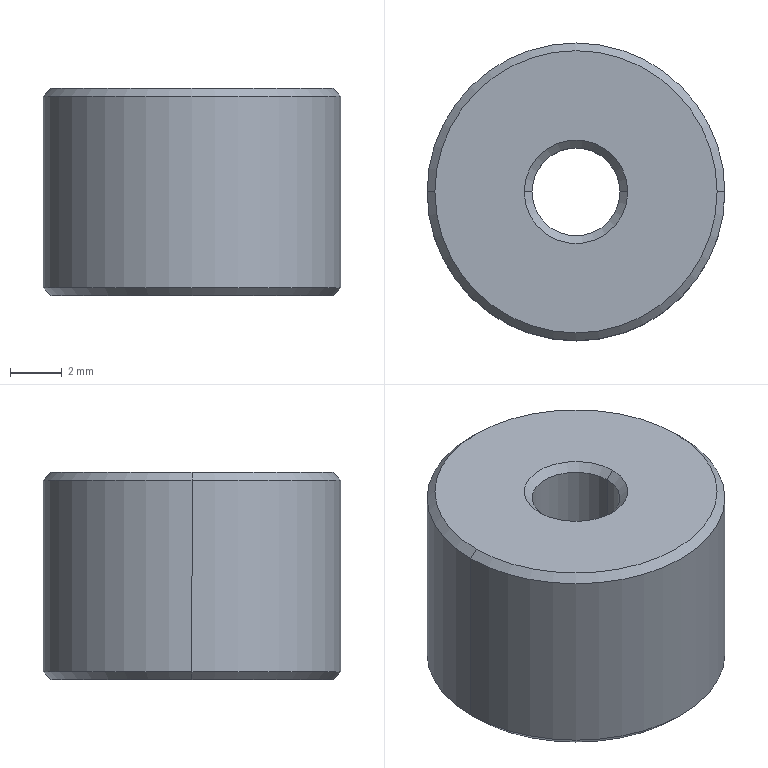Part | STEP file | Guide post cap | 1 solid | 17 faces | box 11.5 x 11.5 x 8 mm | volume 657.251 mm3 | cone 8 | cylinder 6 | plane 3 | commonest cylinder face diameters 3.4 x2 6.5 x2 11.5 x2
STEP:
#1=CARTESIAN_POINT('',(0.,0.,0.));
#2=DIRECTION('',(0.,0.,1.));
#3=DIRECTION('',(1.,0.,0.));
#4=AXIS2_PLACEMENT_3D('',#1,#2,#3);
#5=CARTESIAN_POINT('',(-5.75,0.,7.7));
#6=VERTEX_POINT('',#5);
#7=CARTESIAN_POINT('',(5.75,0.,7.7));
#8=VERTEX_POINT('',#7);
#9=CARTESIAN_POINT('',(0.,0.,7.7));
#10=DIRECTION('',(0.,0.,-1.));
#11=DIRECTION('',(-1.,0.,0.));
#12=AXIS2_PLACEMENT_3D('',#9,#10,#11);
#13=CIRCLE('',#12,5.75);
#14=CARTESIAN_POINT('',(0.,0.,8.));
#15=DIRECTION('',(0.,0.,-1.));
#16=DIRECTION('',(-1.,0.,0.));
#17=AXIS2_PLACEMENT_3D('',#14,#15,#16);
#18=CYLINDRICAL_SURFACE('',#17,5.75);
#19=CARTESIAN_POINT('',(0.,0.3));
#20=DIRECTION('',(1.,0.));
#21=VECTOR('',#20,1.);
#22=LINE('',#19,#21);
#23=(GEOMETRIC_REPRESENTATION_CONTEXT(2)PARAMETRIC_REPRESENTATION_CONTEXT()REPRESENTATION_CONTEXT('',''));
#24=DEFINITIONAL_REPRESENTATION('',(#22),#23);
#25=PCURVE('',#18,#24);
#26=CARTESIAN_POINT('',(0.,0.,7.7));
#27=DIRECTION('',(0.,0.,-1.));
#28=DIRECTION('',(-1.,0.,0.));
#29=AXIS2_PLACEMENT_3D('',#26,#27,#28);
#30=CONICAL_SURFACE('',#29,5.75,0.7854);
#31=CARTESIAN_POINT('',(0.,0.));
#32=DIRECTION('',(1.,0.));
#33=VECTOR('',#32,1.);
#34=LINE('',#31,#33);
#35=(GEOMETRIC_REPRESENTATION_CONTEXT(2)PARAMETRIC_REPRESENTATION_CONTEXT()REPRESENTATION_CONTEXT('',''));
#36=DEFINITIONAL_REPRESENTATION('',(#34),#35);
#37=PCURVE('',#30,#36);
#38=SURFACE_CURVE('',#13,(#25,#37),.PCURVE_S1.);
#39=EDGE_CURVE('',#6,#8,#38,.T.);
#40=ORIENTED_EDGE('',*,*,#39,.T.);
#41=CARTESIAN_POINT('',(5.75,0.,0.3));
#42=VERTEX_POINT('',#41);
#43=CARTESIAN_POINT('',(5.75,0.,8.));
#44=DIRECTION('',(0.,0.,-1.));
#45=VECTOR('',#44,1.);
#46=LINE('',#43,#45);
#47=CARTESIAN_POINT('',(3.142,0.));
#48=DIRECTION('',(0.,1.));
#49=VECTOR('',#48,1.);
#50=LINE('',#47,#49);
#51=(GEOMETRIC_REPRESENTATION_CONTEXT(2)PARAMETRIC_REPRESENTATION_CONTEXT()REPRESENTATION_CONTEXT('',''));
#52=DEFINITIONAL_REPRESENTATION('',(#50),#51);
#53=PCURVE('',#18,#52);
#54=CARTESIAN_POINT('',(0.,0.,8.));
#55=DIRECTION('',(0.,0.,-1.));
#56=DIRECTION('',(-1.,0.,0.));
#57=AXIS2_PLACEMENT_3D('',#54,#55,#56);
#58=CYLINDRICAL_SURFACE('',#57,5.75);
#59=CARTESIAN_POINT('',(3.142,0.));
#60=DIRECTION('',(0.,1.));
#61=VECTOR('',#60,1.);
#62=LINE('',#59,#61);
#63=(GEOMETRIC_REPRESENTATION_CONTEXT(2)PARAMETRIC_REPRESENTATION_CONTEXT()REPRESENTATION_CONTEXT('',''));
#64=DEFINITIONAL_REPRESENTATION('',(#62),#63);
#65=PCURVE('',#58,#64);
#66=SURFACE_CURVE('',#46,(#53,#65),.PCURVE_S1.);
#67=EDGE_CURVE('',#8,#42,#66,.T.);
#68=ORIENTED_EDGE('',*,*,#67,.T.);
#69=CARTESIAN_POINT('',(-5.75,0.,0.3));
#70=VERTEX_POINT('',#69);
#71=CARTESIAN_POINT('',(0.,0.,0.3));
#72=DIRECTION('',(0.,0.,1.));
#73=DIRECTION('',(-1.,0.,0.));
#74=AXIS2_PLACEMENT_3D('',#71,#72,#73);
#75=CIRCLE('',#74,5.75);
#76=CARTESIAN_POINT('',(6.283,7.7));
#77=DIRECTION('',(-1.,0.));
#78=VECTOR('',#77,1.);
#79=LINE('',#76,#78);
#80=(GEOMETRIC_REPRESENTATION_CONTEXT(2)PARAMETRIC_REPRESENTATION_CONTEXT()REPRESENTATION_CONTEXT('',''));
#81=DEFINITIONAL_REPRESENTATION('',(#79),#80);
#82=PCURVE('',#18,#81);
#83=CARTESIAN_POINT('',(0.,0.,0.3));
#84=DIRECTION('',(0.,0.,1.));
#85=DIRECTION('',(1.,0.,0.));
#86=AXIS2_PLACEMENT_3D('',#83,#84,#85);
#87=CONICAL_SURFACE('',#86,5.75,0.7854);
#88=CARTESIAN_POINT('',(-3.142,0.));
#89=DIRECTION('',(1.,0.));
#90=VECTOR('',#89,1.);
#91=LINE('',#88,#90);
#92=(GEOMETRIC_REPRESENTATION_CONTEXT(2)PARAMETRIC_REPRESENTATION_CONTEXT()REPRESENTATION_CONTEXT('',''));
#93=DEFINITIONAL_REPRESENTATION('',(#91),#92);
#94=PCURVE('',#87,#93);
#95=SURFACE_CURVE('',#75,(#82,#94),.PCURVE_S1.);
#96=EDGE_CURVE('',#42,#70,#95,.T.);
#97=ORIENTED_EDGE('',*,*,#96,.T.);
#98=CARTESIAN_POINT('',(-5.75,0.,8.));
#99=DIRECTION('',(0.,0.,-1.));
#100=VECTOR('',#99,1.);
#101=LINE('',#98,#100);
#102=CARTESIAN_POINT('',(0.,0.));
#103=DIRECTION('',(0.,1.));
#104=VECTOR('',#103,1.);
#105=LINE('',#102,#104);
#106=(GEOMETRIC_REPRESENTATION_CONTEXT(2)PARAMETRIC_REPRESENTATION_CONTEXT()REPRESENTATION_CONTEXT('',''));
#107=DEFINITIONAL_REPRESENTATION('',(#105),#106);
#108=PCURVE('',#18,#107);
#109=CARTESIAN_POINT('',(6.283,0.));
#110=DIRECTION('',(0.,1.));
#111=VECTOR('',#110,1.);
#112=LINE('',#109,#111);
#113=(GEOMETRIC_REPRESENTATION_CONTEXT(2)PARAMETRIC_REPRESENTATION_CONTEXT()REPRESENTATION_CONTEXT('',''));
#114=DEFINITIONAL_REPRESENTATION('',(#112),#113);
#115=PCURVE('',#58,#114);
#116=SURFACE_CURVE('',#101,(#108,#115),.PCURVE_S1.);
#117=EDGE_CURVE('',#6,#70,#116,.T.);
#118=ORIENTED_EDGE('',*,*,#117,.F.);
#119=EDGE_LOOP('',(#40,#68,#97,#118));
#120=FACE_BOUND('',#119,.T.);
#121=ADVANCED_FACE('',(#120),#18,.T.);
#122=CARTESIAN_POINT('',(5.45,0.,0.));
#123=VERTEX_POINT('',#122);
#124=CARTESIAN_POINT('',(-5.45,0.,0.));
#125=VERTEX_POINT('',#124);
#126=CARTESIAN_POINT('',(0.,0.,0.));
#127=DIRECTION('',(0.,0.,1.));
#128=DIRECTION('',(1.,0.,0.));
#129=AXIS2_PLACEMENT_3D('',#126,#127,#128);
#130=CIRCLE('',#129,5.45);
#131=CARTESIAN_POINT('',(0.,-0.3));
#132=DIRECTION('',(1.,0.));
#133=VECTOR('',#132,1.);
#134=LINE('',#131,#133);
#135=(GEOMETRIC_REPRESENTATION_CONTEXT(2)PARAMETRIC_REPRESENTATION_CONTEXT()REPRESENTATION_CONTEXT('',''));
#136=DEFINITIONAL_REPRESENTATION('',(#134),#135);
#137=PCURVE('',#87,#136);
#138=CARTESIAN_POINT('',(0.,0.,0.));
#139=DIRECTION('',(0.,0.,1.));
#140=DIRECTION('',(1.,0.,0.));
#141=AXIS2_PLACEMENT_3D('',#138,#139,#140);
#142=PLANE('',#141);
#143=CARTESIAN_POINT('',(0.,0.));
#144=DIRECTION('',(1.,0.));
#145=AXIS2_PLACEMENT_2D('',#143,#144);
#146=CIRCLE('',#145,5.45);
#147=(GEOMETRIC_REPRESENTATION_CONTEXT(2)PARAMETRIC_REPRESENTATION_CONTEXT()REPRESENTATION_CONTEXT('',''));
#148=DEFINITIONAL_REPRESENTATION('',(#146),#147);
#149=PCURVE('',#142,#148);
#150=SURFACE_CURVE('',#130,(#137,#149),.PCURVE_S1.);
#151=EDGE_CURVE('',#123,#125,#150,.T.);
#152=ORIENTED_EDGE('',*,*,#151,.T.);
#153=CARTESIAN_POINT('',(-5.75,0.,0.3));
#154=DIRECTION('',(-0.7071,0.,0.7071));
#155=VECTOR('',#154,1.);
#156=LINE('',#153,#155);
#157=CARTESIAN_POINT('',(3.142,0.));
#158=DIRECTION('',(0.,1.));
#159=VECTOR('',#158,1.);
#160=LINE('',#157,#159);
#161=(GEOMETRIC_REPRESENTATION_CONTEXT(2)PARAMETRIC_REPRESENTATION_CONTEXT()REPRESENTATION_CONTEXT('',''));
#162=DEFINITIONAL_REPRESENTATION('',(#160),#161);
#163=PCURVE('',#87,#162);
#164=CARTESIAN_POINT('',(0.,0.,0.3));
#165=DIRECTION('',(0.,0.,1.));
#166=DIRECTION('',(1.,0.,0.));
#167=AXIS2_PLACEMENT_3D('',#164,#165,#166);
#168=CONICAL_SURFACE('',#167,5.75,0.7854);
#169=CARTESIAN_POINT('',(3.142,0.));
#170=DIRECTION('',(0.,1.));
#171=VECTOR('',#170,1.);
#172=LINE('',#169,#171);
#173=(GEOMETRIC_REPRESENTATION_CONTEXT(2)PARAMETRIC_REPRESENTATION_CONTEXT()REPRESENTATION_CONTEXT('',''));
#174=DEFINITIONAL_REPRESENTATION('',(#172),#173);
#175=PCURVE('',#168,#174);
#176=SURFACE_CURVE('',#156,(#163,#175),.PCURVE_S1.);
#177=EDGE_CURVE('',#125,#70,#176,.T.);
#178=ORIENTED_EDGE('',*,*,#177,.T.);
#179=ORIENTED_EDGE('',*,*,#96,.F.);
#180=CARTESIAN_POINT('',(5.75,0.,0.3));
#181=DIRECTION('',(0.7071,0.,0.7071));
#182=VECTOR('',#181,1.);
#183=LINE('',#180,#182);
#184=CARTESIAN_POINT('',(0.,0.));
#185=DIRECTION('',(0.,1.));
#186=VECTOR('',#185,1.);
#187=LINE('',#184,#186);
#188=(GEOMETRIC_REPRESENTATION_CONTEXT(2)PARAMETRIC_REPRESENTATION_CONTEXT()REPRESENTATION_CONTEXT('',''));
#189=DEFINITIONAL_REPRESENTATION('',(#187),#188);
#190=PCURVE('',#87,#189);
#191=CARTESIAN_POINT('',(6.283,0.));
#192=DIRECTION('',(0.,1.));
#193=VECTOR('',#192,1.);
#194=LINE('',#191,#193);
#195=(GEOMETRIC_REPRESENTATION_CONTEXT(2)PARAMETRIC_REPRESENTATION_CONTEXT()REPRESENTATION_CONTEXT('',''));
#196=DEFINITIONAL_REPRESENTATION('',(#194),#195);
#197=PCURVE('',#168,#196);
#198=SURFACE_CURVE('',#183,(#190,#197),.PCURVE_S1.);
#199=EDGE_CURVE('',#123,#42,#198,.T.);
#200=ORIENTED_EDGE('',*,*,#199,.F.);
#201=EDGE_LOOP('',(#152,#178,#179,#200));
#202=FACE_BOUND('',#201,.T.);
#203=ADVANCED_FACE('',(#202),#87,.T.);
#204=CARTESIAN_POINT('',(-5.45,0.,8.));
#205=VERTEX_POINT('',#204);
#206=CARTESIAN_POINT('',(5.45,0.,8.));
#207=VERTEX_POINT('',#206);
#208=CARTESIAN_POINT('',(0.,0.,8.));
#209=DIRECTION('',(0.,0.,-1.));
#210=DIRECTION('',(-1.,0.,0.));
#211=AXIS2_PLACEMENT_3D('',#208,#209,#210);
#212=CIRCLE('',#211,5.45);
#213=CARTESIAN_POINT('',(0.,-0.3));
#214=DIRECTION('',(1.,0.));
#215=VECTOR('',#214,1.);
#216=LINE('',#213,#215);
#217=(GEOMETRIC_REPRESENTATION_CONTEXT(2)PARAMETRIC_REPRESENTATION_CONTEXT()REPRESENTATION_CONTEXT('',''));
#218=DEFINITIONAL_REPRESENTATION('',(#216),#217);
#219=PCURVE('',#30,#218);
#220=CARTESIAN_POINT('',(0.,0.,8.));
#221=DIRECTION('',(0.,0.,1.));
#222=DIRECTION('',(1.,0.,0.));
#223=AXIS2_PLACEMENT_3D('',#220,#221,#222);
#224=PLANE('',#223);
#225=CARTESIAN_POINT('',(-5.45,0.));
#226=CARTESIAN_POINT('',(-5.45,9.44));
#227=CARTESIAN_POINT('',(2.725,4.72));
#228=CARTESIAN_POINT('',(10.9,0.));
#229=CARTESIAN_POINT('',(2.725,-4.72));
#230=CARTESIAN_POINT('',(-5.45,-9.44));
#231=CARTESIAN_POINT('',(-5.45,0.));
#232=(BOUNDED_CURVE()B_SPLINE_CURVE(2,(#225,#226,#227,#228,#229,#230,#231),.UNSPECIFIED.,.T.,.F.)B_SPLINE_CURVE_WITH_KNOTS((1,2,2,2,2,1),(-2.094,0.,2.094,4.189,6.283,8.378),.UNSPECIFIED.)CURVE()GEOMETRIC_REPRESENTATION_ITEM()RATIONAL_B_SPLINE_CURVE((1.,0.5,1.,0.5,1.,0.5,1.))REPRESENTATION_ITEM(''));
#233=(GEOMETRIC_REPRESENTATION_CONTEXT(2)PARAMETRIC_REPRESENTATION_CONTEXT()REPRESENTATION_CONTEXT('',''));
#234=DEFINITIONAL_REPRESENTATION('',(#232),#233);
#235=PCURVE('',#224,#234);
#236=SURFACE_CURVE('',#212,(#219,#235),.PCURVE_S1.);
#237=EDGE_CURVE('',#205,#207,#236,.T.);
#238=ORIENTED_EDGE('',*,*,#237,.T.);
#239=CARTESIAN_POINT('',(5.75,0.,7.7));
#240=DIRECTION('',(0.7071,0.,-0.7071));
#241=VECTOR('',#240,1.);
#242=LINE('',#239,#241);
#243=CARTESIAN_POINT('',(3.142,0.));
#244=DIRECTION('',(0.,1.));
#245=VECTOR('',#244,1.);
#246=LINE('',#243,#245);
#247=(GEOMETRIC_REPRESENTATION_CONTEXT(2)PARAMETRIC_REPRESENTATION_CONTEXT()REPRESENTATION_CONTEXT('',''));
#248=DEFINITIONAL_REPRESENTATION('',(#246),#247);
#249=PCURVE('',#30,#248);
#250=CARTESIAN_POINT('',(0.,0.,7.7));
#251=DIRECTION('',(0.,0.,-1.));
#252=DIRECTION('',(-1.,0.,0.));
#253=AXIS2_PLACEMENT_3D('',#250,#251,#252);
#254=CONICAL_SURFACE('',#253,5.75,0.7854);
#255=CARTESIAN_POINT('',(3.142,0.));
#256=DIRECTION('',(0.,1.));
#257=VECTOR('',#256,1.);
#258=LINE('',#255,#257);
#259=(GEOMETRIC_REPRESENTATION_CONTEXT(2)PARAMETRIC_REPRESENTATION_CONTEXT()REPRESENTATION_CONTEXT('',''));
#260=DEFINITIONAL_REPRESENTATION('',(#258),#259);
#261=PCURVE('',#254,#260);
#262=SURFACE_CURVE('',#242,(#249,#261),.PCURVE_S1.);
#263=EDGE_CURVE('',#207,#8,#262,.T.);
#264=ORIENTED_EDGE('',*,*,#263,.T.);
#265=ORIENTED_EDGE('',*,*,#39,.F.);
#266=CARTESIAN_POINT('',(-5.75,0.,7.7));
#267=DIRECTION('',(-0.7071,0.,-0.7071));
#268=VECTOR('',#267,1.);
#269=LINE('',#266,#268);
#270=CARTESIAN_POINT('',(0.,0.));
#271=DIRECTION('',(0.,1.));
#272=VECTOR('',#271,1.);
#273=LINE('',#270,#272);
#274=(GEOMETRIC_REPRESENTATION_CONTEXT(2)PARAMETRIC_REPRESENTATION_CONTEXT()REPRESENTATION_CONTEXT('',''));
#275=DEFINITIONAL_REPRESENTATION('',(#273),#274);
#276=PCURVE('',#30,#275);
#277=CARTESIAN_POINT('',(6.283,0.));
#278=DIRECTION('',(0.,1.));
#279=VECTOR('',#278,1.);
#280=LINE('',#277,#279);
#281=(GEOMETRIC_REPRESENTATION_CONTEXT(2)PARAMETRIC_REPRESENTATION_CONTEXT()REPRESENTATION_CONTEXT('',''));
#282=DEFINITIONAL_REPRESENTATION('',(#280),#281);
#283=PCURVE('',#254,#282);
#284=SURFACE_CURVE('',#269,(#276,#283),.PCURVE_S1.);
#285=EDGE_CURVE('',#205,#6,#284,.T.);
#286=ORIENTED_EDGE('',*,*,#285,.F.);
#287=EDGE_LOOP('',(#238,#264,#265,#286));
#288=FACE_BOUND('',#287,.T.);
#289=ADVANCED_FACE('',(#288),#30,.T.);
#290=CARTESIAN_POINT('',(-3.25,0.,0.3));
#291=VERTEX_POINT('',#290);
#292=CARTESIAN_POINT('',(-3.55,0.,0.));
#293=VERTEX_POINT('',#292);
#294=CARTESIAN_POINT('',(-3.55,0.,0.));
#295=DIRECTION('',(-0.7071,0.,-0.7071));
#296=VECTOR('',#295,1.);
#297=LINE('',#294,#296);
#298=CARTESIAN_POINT('',(0.,0.,0.));
#299=DIRECTION('',(0.,0.,-1.));
#300=DIRECTION('',(-1.,0.,0.));
#301=AXIS2_PLACEMENT_3D('',#298,#299,#300);
#302=CONICAL_SURFACE('',#301,3.55,0.7854);
#303=CARTESIAN_POINT('',(6.283,0.));
#304=DIRECTION('',(0.,1.));
#305=VECTOR('',#304,1.);
#306=LINE('',#303,#305);
#307=(GEOMETRIC_REPRESENTATION_CONTEXT(2)PARAMETRIC_REPRESENTATION_CONTEXT()REPRESENTATION_CONTEXT('',''));
#308=DEFINITIONAL_REPRESENTATION('',(#306),#307);
#309=PCURVE('',#302,#308);
#310=CARTESIAN_POINT('',(0.,0.,0.));
#311=DIRECTION('',(0.,0.,-1.));
#312=DIRECTION('',(-1.,0.,0.));
#313=AXIS2_PLACEMENT_3D('',#310,#311,#312);
#314=CONICAL_SURFACE('',#313,3.55,0.7854);
#315=CARTESIAN_POINT('',(0.,0.));
#316=DIRECTION('',(0.,1.));
#317=VECTOR('',#316,1.);
#318=LINE('',#315,#317);
#319=(GEOMETRIC_REPRESENTATION_CONTEXT(2)PARAMETRIC_REPRESENTATION_CONTEXT()REPRESENTATION_CONTEXT('',''));
#320=DEFINITIONAL_REPRESENTATION('',(#318),#319);
#321=PCURVE('',#314,#320);
#322=SURFACE_CURVE('',#297,(#309,#321),.PCURVE_S1.);
#323=EDGE_CURVE('',#291,#293,#322,.T.);
#324=ORIENTED_EDGE('',*,*,#323,.T.);
#325=CARTESIAN_POINT('',(3.55,0.,0.));
#326=VERTEX_POINT('',#325);
#327=CARTESIAN_POINT('',(0.,0.,0.));
#328=DIRECTION('',(0.,0.,-1.));
#329=DIRECTION('',(-1.,0.,0.));
#330=AXIS2_PLACEMENT_3D('',#327,#328,#329);
#331=CIRCLE('',#330,3.55);
#332=CARTESIAN_POINT('',(0.,0.));
#333=DIRECTION('',(1.,0.));
#334=VECTOR('',#333,1.);
#335=LINE('',#332,#334);
#336=(GEOMETRIC_REPRESENTATION_CONTEXT(2)PARAMETRIC_REPRESENTATION_CONTEXT()REPRESENTATION_CONTEXT('',''));
#337=DEFINITIONAL_REPRESENTATION('',(#335),#336);
#338=PCURVE('',#302,#337);
#339=CARTESIAN_POINT('',(-3.55,0.));
#340=CARTESIAN_POINT('',(-3.55,6.149));
#341=CARTESIAN_POINT('',(1.775,3.074));
#342=CARTESIAN_POINT('',(7.1,0.));
#343=CARTESIAN_POINT('',(1.775,-3.074));
#344=CARTESIAN_POINT('',(-3.55,-6.149));
#345=CARTESIAN_POINT('',(-3.55,0.));
#346=(BOUNDED_CURVE()B_SPLINE_CURVE(2,(#339,#340,#341,#342,#343,#344,#345),.UNSPECIFIED.,.T.,.F.)B_SPLINE_CURVE_WITH_KNOTS((1,2,2,2,2,1),(-2.094,0.,2.094,4.189,6.283,8.378),.UNSPECIFIED.)CURVE()GEOMETRIC_REPRESENTATION_ITEM()RATIONAL_B_SPLINE_CURVE((1.,0.5,1.,0.5,1.,0.5,1.))REPRESENTATION_ITEM(''));
#347=(GEOMETRIC_REPRESENTATION_CONTEXT(2)PARAMETRIC_REPRESENTATION_CONTEXT()REPRESENTATION_CONTEXT('',''));
#348=DEFINITIONAL_REPRESENTATION('',(#346),#347);
#349=PCURVE('',#142,#348);
#350=SURFACE_CURVE('',#331,(#338,#349),.PCURVE_S1.);
#351=EDGE_CURVE('',#326,#293,#350,.T.);
#352=ORIENTED_EDGE('',*,*,#351,.F.);
#353=CARTESIAN_POINT('',(3.25,0.,0.3));
#354=VERTEX_POINT('',#353);
#355=CARTESIAN_POINT('',(3.55,0.,0.));
#356=DIRECTION('',(0.7071,0.,-0.7071));
#357=VECTOR('',#356,1.);
#358=LINE('',#355,#357);
#359=CARTESIAN_POINT('',(3.142,0.));
#360=DIRECTION('',(0.,1.));
#361=VECTOR('',#360,1.);
#362=LINE('',#359,#361);
#363=(GEOMETRIC_REPRESENTATION_CONTEXT(2)PARAMETRIC_REPRESENTATION_CONTEXT()REPRESENTATION_CONTEXT('',''));
#364=DEFINITIONAL_REPRESENTATION('',(#362),#363);
#365=PCURVE('',#302,#364);
#366=CARTESIAN_POINT('',(3.142,0.));
#367=DIRECTION('',(0.,1.));
#368=VECTOR('',#367,1.);
#369=LINE('',#366,#368);
#370=(GEOMETRIC_REPRESENTATION_CONTEXT(2)PARAMETRIC_REPRESENTATION_CONTEXT()REPRESENTATION_CONTEXT('',''));
#371=DEFINITIONAL_REPRESENTATION('',(#369),#370);
#372=PCURVE('',#314,#371);
#373=SURFACE_CURVE('',#358,(#365,#372),.PCURVE_S1.);
#374=EDGE_CURVE('',#354,#326,#373,.T.);
#375=ORIENTED_EDGE('',*,*,#374,.F.);
#376=CARTESIAN_POINT('',(0.,0.,0.3));
#377=DIRECTION('',(0.,0.,-1.));
#378=DIRECTION('',(-1.,0.,0.));
#379=AXIS2_PLACEMENT_3D('',#376,#377,#378);
#380=CIRCLE('',#379,3.25);
#381=CARTESIAN_POINT('',(0.,-0.3));
#382=DIRECTION('',(1.,0.));
#383=VECTOR('',#382,1.);
#384=LINE('',#381,#383);
#385=(GEOMETRIC_REPRESENTATION_CONTEXT(2)PARAMETRIC_REPRESENTATION_CONTEXT()REPRESENTATION_CONTEXT('',''));
#386=DEFINITIONAL_REPRESENTATION('',(#384),#385);
#387=PCURVE('',#302,#386);
#388=CARTESIAN_POINT('',(0.,0.,0.));
#389=DIRECTION('',(0.,0.,-1.));
#390=DIRECTION('',(-1.,0.,0.));
#391=AXIS2_PLACEMENT_3D('',#388,#389,#390);
#392=CYLINDRICAL_SURFACE('',#391,3.25);
#393=CARTESIAN_POINT('',(0.,-0.3));
#394=DIRECTION('',(1.,0.));
#395=VECTOR('',#394,1.);
#396=LINE('',#393,#395);
#397=(GEOMETRIC_REPRESENTATION_CONTEXT(2)PARAMETRIC_REPRESENTATION_CONTEXT()REPRESENTATION_CONTEXT('',''));
#398=DEFINITIONAL_REPRESENTATION('',(#396),#397);
#399=PCURVE('',#392,#398);
#400=SURFACE_CURVE('',#380,(#387,#399),.PCURVE_S1.);
#401=EDGE_CURVE('',#354,#291,#400,.T.);
#402=ORIENTED_EDGE('',*,*,#401,.T.);
#403=EDGE_LOOP('',(#324,#352,#375,#402));
#404=FACE_BOUND('',#403,.F.);
#405=ADVANCED_FACE('',(#404),#302,.F.);
#406=CARTESIAN_POINT('',(1.7,0.,7.7));
#407=VERTEX_POINT('',#406);
#408=CARTESIAN_POINT('',(2.,0.,8.));
#409=VERTEX_POINT('',#408);
#410=CARTESIAN_POINT('',(2.,0.,8.));
#411=DIRECTION('',(0.7071,0.,0.7071));
#412=VECTOR('',#411,1.);
#413=LINE('',#410,#412);
#414=CARTESIAN_POINT('',(0.,0.,8.));
#415=DIRECTION('',(0.,0.,1.));
#416=DIRECTION('',(1.,0.,0.));
#417=AXIS2_PLACEMENT_3D('',#414,#415,#416);
#418=CONICAL_SURFACE('',#417,2.,0.7854);
#419=CARTESIAN_POINT('',(6.283,0.));
#420=DIRECTION('',(0.,1.));
#421=VECTOR('',#420,1.);
#422=LINE('',#419,#421);
#423=(GEOMETRIC_REPRESENTATION_CONTEXT(2)PARAMETRIC_REPRESENTATION_CONTEXT()REPRESENTATION_CONTEXT('',''));
#424=DEFINITIONAL_REPRESENTATION('',(#422),#423);
#425=PCURVE('',#418,#424);
#426=CARTESIAN_POINT('',(0.,0.,8.));
#427=DIRECTION('',(0.,0.,1.));
#428=DIRECTION('',(1.,0.,0.));
#429=AXIS2_PLACEMENT_3D('',#426,#427,#428);
#430=CONICAL_SURFACE('',#429,2.,0.7854);
#431=CARTESIAN_POINT('',(0.,0.));
#432=DIRECTION('',(0.,1.));
#433=VECTOR('',#432,1.);
#434=LINE('',#431,#433);
#435=(GEOMETRIC_REPRESENTATION_CONTEXT(2)PARAMETRIC_REPRESENTATION_CONTEXT()REPRESENTATION_CONTEXT('',''));
#436=DEFINITIONAL_REPRESENTATION('',(#434),#435);
#437=PCURVE('',#430,#436);
#438=SURFACE_CURVE('',#413,(#425,#437),.PCURVE_S1.);
#439=EDGE_CURVE('',#407,#409,#438,.T.);
#440=ORIENTED_EDGE('',*,*,#439,.T.);
#441=CARTESIAN_POINT('',(-2.,0.,8.));
#442=VERTEX_POINT('',#441);
#443=CARTESIAN_POINT('',(0.,0.,8.));
#444=DIRECTION('',(0.,0.,-1.));
#445=DIRECTION('',(1.,0.,0.));
#446=AXIS2_PLACEMENT_3D('',#443,#444,#445);
#447=CIRCLE('',#446,2.);
#448=CARTESIAN_POINT('',(6.283,0.));
#449=DIRECTION('',(-1.,0.));
#450=VECTOR('',#449,1.);
#451=LINE('',#448,#450);
#452=(GEOMETRIC_REPRESENTATION_CONTEXT(2)PARAMETRIC_REPRESENTATION_CONTEXT()REPRESENTATION_CONTEXT('',''));
#453=DEFINITIONAL_REPRESENTATION('',(#451),#452);
#454=PCURVE('',#418,#453);
#455=CARTESIAN_POINT('',(2.,0.));
#456=CARTESIAN_POINT('',(2.,-3.464));
#457=CARTESIAN_POINT('',(-1.,-1.732));
#458=CARTESIAN_POINT('',(-4.,0.));
#459=CARTESIAN_POINT('',(-1.,1.732));
#460=CARTESIAN_POINT('',(2.,3.464));
#461=CARTESIAN_POINT('',(2.,0.));
#462=(BOUNDED_CURVE()B_SPLINE_CURVE(2,(#455,#456,#457,#458,#459,#460,#461),.UNSPECIFIED.,.T.,.F.)B_SPLINE_CURVE_WITH_KNOTS((1,2,2,2,2,1),(-2.094,0.,2.094,4.189,6.283,8.378),.UNSPECIFIED.)CURVE()GEOMETRIC_REPRESENTATION_ITEM()RATIONAL_B_SPLINE_CURVE((1.,0.5,1.,0.5,1.,0.5,1.))REPRESENTATION_ITEM(''));
#463=(GEOMETRIC_REPRESENTATION_CONTEXT(2)PARAMETRIC_REPRESENTATION_CONTEXT()REPRESENTATION_CONTEXT('',''));
#464=DEFINITIONAL_REPRESENTATION('',(#462),#463);
#465=PCURVE('',#224,#464);
#466=SURFACE_CURVE('',#447,(#454,#465),.PCURVE_S1.);
#467=EDGE_CURVE('',#409,#442,#466,.T.);
#468=ORIENTED_EDGE('',*,*,#467,.T.);
#469=CARTESIAN_POINT('',(-1.7,0.,7.7));
#470=VERTEX_POINT('',#469);
#471=CARTESIAN_POINT('',(-2.,0.,8.));
#472=DIRECTION('',(-0.7071,0.,0.7071));
#473=VECTOR('',#472,1.);
#474=LINE('',#471,#473);
#475=CARTESIAN_POINT('',(3.142,0.));
#476=DIRECTION('',(0.,1.));
#477=VECTOR('',#476,1.);
#478=LINE('',#475,#477);
#479=(GEOMETRIC_REPRESENTATION_CONTEXT(2)PARAMETRIC_REPRESENTATION_CONTEXT()REPRESENTATION_CONTEXT('',''));
#480=DEFINITIONAL_REPRESENTATION('',(#478),#479);
#481=PCURVE('',#418,#480);
#482=CARTESIAN_POINT('',(3.142,0.));
#483=DIRECTION('',(0.,1.));
#484=VECTOR('',#483,1.);
#485=LINE('',#482,#484);
#486=(GEOMETRIC_REPRESENTATION_CONTEXT(2)PARAMETRIC_REPRESENTATION_CONTEXT()REPRESENTATION_CONTEXT('',''));
#487=DEFINITIONAL_REPRESENTATION('',(#485),#486);
#488=PCURVE('',#430,#487);
#489=SURFACE_CURVE('',#474,(#481,#488),.PCURVE_S1.);
#490=EDGE_CURVE('',#470,#442,#489,.T.);
#491=ORIENTED_EDGE('',*,*,#490,.F.);
#492=CARTESIAN_POINT('',(0.,0.,7.7));
#493=DIRECTION('',(0.,0.,1.));
#494=DIRECTION('',(1.,0.,0.));
#495=AXIS2_PLACEMENT_3D('',#492,#493,#494);
#496=CIRCLE('',#495,1.7);
#497=CARTESIAN_POINT('',(0.,-0.3));
#498=DIRECTION('',(1.,0.));
#499=VECTOR('',#498,1.);
#500=LINE('',#497,#499);
#501=(GEOMETRIC_REPRESENTATION_CONTEXT(2)PARAMETRIC_REPRESENTATION_CONTEXT()REPRESENTATION_CONTEXT('',''));
#502=DEFINITIONAL_REPRESENTATION('',(#500),#501);
#503=PCURVE('',#418,#502);
#504=CARTESIAN_POINT('',(0.,0.,0.));
#505=DIRECTION('',(0.,0.,-1.));
#506=DIRECTION('',(-1.,0.,0.));
#507=AXIS2_PLACEMENT_3D('',#504,#505,#506);
#508=CYLINDRICAL_SURFACE('',#507,1.7);
#509=CARTESIAN_POINT('',(9.425,-7.7));
#510=DIRECTION('',(-1.,0.));
#511=VECTOR('',#510,1.);
#512=LINE('',#509,#511);
#513=(GEOMETRIC_REPRESENTATION_CONTEXT(2)PARAMETRIC_REPRESENTATION_CONTEXT()REPRESENTATION_CONTEXT('',''));
#514=DEFINITIONAL_REPRESENTATION('',(#512),#513);
#515=PCURVE('',#508,#514);
#516=SURFACE_CURVE('',#496,(#503,#515),.PCURVE_S1.);
#517=EDGE_CURVE('',#470,#407,#516,.T.);
#518=ORIENTED_EDGE('',*,*,#517,.T.);
#519=EDGE_LOOP('',(#440,#468,#491,#518));
#520=FACE_BOUND('',#519,.F.);
#521=ADVANCED_FACE('',(#520),#418,.F.);
#522=CARTESIAN_POINT('',(-3.25,0.,4.));
#523=VERTEX_POINT('',#522);
#524=CARTESIAN_POINT('',(-3.25,0.,0.));
#525=DIRECTION('',(0.,0.,-1.));
#526=VECTOR('',#525,1.);
#527=LINE('',#524,#526);
#528=CARTESIAN_POINT('',(6.283,0.));
#529=DIRECTION('',(0.,1.));
#530=VECTOR('',#529,1.);
#531=LINE('',#528,#530);
#532=(GEOMETRIC_REPRESENTATION_CONTEXT(2)PARAMETRIC_REPRESENTATION_CONTEXT()REPRESENTATION_CONTEXT('',''));
#533=DEFINITIONAL_REPRESENTATION('',(#531),#532);
#534=PCURVE('',#392,#533);
#535=CARTESIAN_POINT('',(0.,0.,0.));
#536=DIRECTION('',(0.,0.,-1.));
#537=DIRECTION('',(-1.,0.,0.));
#538=AXIS2_PLACEMENT_3D('',#535,#536,#537);
#539=CYLINDRICAL_SURFACE('',#538,3.25);
#540=CARTESIAN_POINT('',(0.,0.));
#541=DIRECTION('',(0.,1.));
#542=VECTOR('',#541,1.);
#543=LINE('',#540,#542);
#544=(GEOMETRIC_REPRESENTATION_CONTEXT(2)PARAMETRIC_REPRESENTATION_CONTEXT()REPRESENTATION_CONTEXT('',''));
#545=DEFINITIONAL_REPRESENTATION('',(#543),#544);
#546=PCURVE('',#539,#545);
#547=SURFACE_CURVE('',#527,(#534,#546),.PCURVE_S1.);
#548=EDGE_CURVE('',#523,#291,#547,.T.);
#549=ORIENTED_EDGE('',*,*,#548,.T.);
#550=ORIENTED_EDGE('',*,*,#401,.F.);
#551=CARTESIAN_POINT('',(3.25,0.,4.));
#552=VERTEX_POINT('',#551);
#553=CARTESIAN_POINT('',(3.25,0.,0.));
#554=DIRECTION('',(0.,0.,-1.));
#555=VECTOR('',#554,1.);
#556=LINE('',#553,#555);
#557=CARTESIAN_POINT('',(3.142,0.));
#558=DIRECTION('',(0.,1.));
#559=VECTOR('',#558,1.);
#560=LINE('',#557,#559);
#561=(GEOMETRIC_REPRESENTATION_CONTEXT(2)PARAMETRIC_REPRESENTATION_CONTEXT()REPRESENTATION_CONTEXT('',''));
#562=DEFINITIONAL_REPRESENTATION('',(#560),#561);
#563=PCURVE('',#392,#562);
#564=CARTESIAN_POINT('',(3.142,0.));
#565=DIRECTION('',(0.,1.));
#566=VECTOR('',#565,1.);
#567=LINE('',#564,#566);
#568=(GEOMETRIC_REPRESENTATION_CONTEXT(2)PARAMETRIC_REPRESENTATION_CONTEXT()REPRESENTATION_CONTEXT('',''));
#569=DEFINITIONAL_REPRESENTATION('',(#567),#568);
#570=PCURVE('',#539,#569);
#571=SURFACE_CURVE('',#556,(#563,#570),.PCURVE_S1.);
#572=EDGE_CURVE('',#552,#354,#571,.T.);
#573=ORIENTED_EDGE('',*,*,#572,.F.);
#574=CARTESIAN_POINT('',(0.,0.,4.));
#575=DIRECTION('',(0.,0.,-1.));
#576=DIRECTION('',(-1.,0.,0.));
#577=AXIS2_PLACEMENT_3D('',#574,#575,#576);
#578=CIRCLE('',#577,3.25);
#579=CARTESIAN_POINT('',(0.,-4.));
#580=DIRECTION('',(1.,0.));
#581=VECTOR('',#580,1.);
#582=LINE('',#579,#581);
#583=(GEOMETRIC_REPRESENTATION_CONTEXT(2)PARAMETRIC_REPRESENTATION_CONTEXT()REPRESENTATION_CONTEXT('',''));
#584=DEFINITIONAL_REPRESENTATION('',(#582),#583);
#585=PCURVE('',#392,#584);
#586=CARTESIAN_POINT('',(1.7,0.,4.));
#587=DIRECTION('',(0.,0.,1.));
#588=DIRECTION('',(1.,0.,0.));
#589=AXIS2_PLACEMENT_3D('',#586,#587,#588);
#590=PLANE('',#589);
#591=CARTESIAN_POINT('',(-4.95,0.));
#592=CARTESIAN_POINT('',(-4.95,5.629));
#593=CARTESIAN_POINT('',(-0.075,2.815));
#594=CARTESIAN_POINT('',(4.8,0.));
#595=CARTESIAN_POINT('',(-0.075,-2.815));
#596=CARTESIAN_POINT('',(-4.95,-5.629));
#597=CARTESIAN_POINT('',(-4.95,0.));
#598=(BOUNDED_CURVE()B_SPLINE_CURVE(2,(#591,#592,#593,#594,#595,#596,#597),.UNSPECIFIED.,.T.,.F.)B_SPLINE_CURVE_WITH_KNOTS((1,2,2,2,2,1),(-2.094,0.,2.094,4.189,6.283,8.378),.UNSPECIFIED.)CURVE()GEOMETRIC_REPRESENTATION_ITEM()RATIONAL_B_SPLINE_CURVE((1.,0.5,1.,0.5,1.,0.5,1.))REPRESENTATION_ITEM(''));
#599=(GEOMETRIC_REPRESENTATION_CONTEXT(2)PARAMETRIC_REPRESENTATION_CONTEXT()REPRESENTATION_CONTEXT('',''));
#600=DEFINITIONAL_REPRESENTATION('',(#598),#599);
#601=PCURVE('',#590,#600);
#602=SURFACE_CURVE('',#578,(#585,#601),.PCURVE_S1.);
#603=EDGE_CURVE('',#552,#523,#602,.T.);
#604=ORIENTED_EDGE('',*,*,#603,.T.);
#605=EDGE_LOOP('',(#549,#550,#573,#604));
#606=FACE_BOUND('',#605,.F.);
#607=ADVANCED_FACE('',(#606),#392,.F.);
#608=CARTESIAN_POINT('',(-1.7,0.,4.));
#609=VERTEX_POINT('',#608);
#610=CARTESIAN_POINT('',(-1.7,0.,0.));
#611=DIRECTION('',(0.,0.,-1.));
#612=VECTOR('',#611,1.);
#613=LINE('',#610,#612);
#614=CARTESIAN_POINT('',(6.283,0.));
#615=DIRECTION('',(0.,1.));
#616=VECTOR('',#615,1.);
#617=LINE('',#614,#616);
#618=(GEOMETRIC_REPRESENTATION_CONTEXT(2)PARAMETRIC_REPRESENTATION_CONTEXT()REPRESENTATION_CONTEXT('',''));
#619=DEFINITIONAL_REPRESENTATION('',(#617),#618);
#620=PCURVE('',#508,#619);
#621=CARTESIAN_POINT('',(0.,0.,0.));
#622=DIRECTION('',(0.,0.,-1.));
#623=DIRECTION('',(-1.,0.,0.));
#624=AXIS2_PLACEMENT_3D('',#621,#622,#623);
#625=CYLINDRICAL_SURFACE('',#624,1.7);
#626=CARTESIAN_POINT('',(0.,0.));
#627=DIRECTION('',(0.,1.));
#628=VECTOR('',#627,1.);
#629=LINE('',#626,#628);
#630=(GEOMETRIC_REPRESENTATION_CONTEXT(2)PARAMETRIC_REPRESENTATION_CONTEXT()REPRESENTATION_CONTEXT('',''));
#631=DEFINITIONAL_REPRESENTATION('',(#629),#630);
#632=PCURVE('',#625,#631);
#633=SURFACE_CURVE('',#613,(#620,#632),.PCURVE_S1.);
#634=EDGE_CURVE('',#470,#609,#633,.T.);
#635=ORIENTED_EDGE('',*,*,#634,.T.);
#636=CARTESIAN_POINT('',(1.7,0.,4.));
#637=VERTEX_POINT('',#636);
#638=CARTESIAN_POINT('',(0.,0.,4.));
#639=DIRECTION('',(0.,0.,1.));
#640=DIRECTION('',(-1.,0.,0.));
#641=AXIS2_PLACEMENT_3D('',#638,#639,#640);
#642=CIRCLE('',#641,1.7);
#643=CARTESIAN_POINT('',(6.283,-4.));
#644=DIRECTION('',(-1.,0.));
#645=VECTOR('',#644,1.);
#646=LINE('',#643,#645);
#647=(GEOMETRIC_REPRESENTATION_CONTEXT(2)PARAMETRIC_REPRESENTATION_CONTEXT()REPRESENTATION_CONTEXT('',''));
#648=DEFINITIONAL_REPRESENTATION('',(#646),#647);
#649=PCURVE('',#508,#648);
#650=CARTESIAN_POINT('',(-1.7,0.));
#651=DIRECTION('',(-1.,0.));
#652=AXIS2_PLACEMENT_2D('',#650,#651);
#653=CIRCLE('',#652,1.7);
#654=(GEOMETRIC_REPRESENTATION_CONTEXT(2)PARAMETRIC_REPRESENTATION_CONTEXT()REPRESENTATION_CONTEXT('',''));
#655=DEFINITIONAL_REPRESENTATION('',(#653),#654);
#656=PCURVE('',#590,#655);
#657=SURFACE_CURVE('',#642,(#649,#656),.PCURVE_S1.);
#658=EDGE_CURVE('',#609,#637,#657,.T.);
#659=ORIENTED_EDGE('',*,*,#658,.T.);
#660=CARTESIAN_POINT('',(1.7,0.,0.));
#661=DIRECTION('',(0.,0.,-1.));
#662=VECTOR('',#661,1.);
#663=LINE('',#660,#662);
#664=CARTESIAN_POINT('',(3.142,0.));
#665=DIRECTION('',(0.,1.));
#666=VECTOR('',#665,1.);
#667=LINE('',#664,#666);
#668=(GEOMETRIC_REPRESENTATION_CONTEXT(2)PARAMETRIC_REPRESENTATION_CONTEXT()REPRESENTATION_CONTEXT('',''));
#669=DEFINITIONAL_REPRESENTATION('',(#667),#668);
#670=PCURVE('',#508,#669);
#671=CARTESIAN_POINT('',(3.142,0.));
#672=DIRECTION('',(0.,1.));
#673=VECTOR('',#672,1.);
#674=LINE('',#671,#673);
#675=(GEOMETRIC_REPRESENTATION_CONTEXT(2)PARAMETRIC_REPRESENTATION_CONTEXT()REPRESENTATION_CONTEXT('',''));
#676=DEFINITIONAL_REPRESENTATION('',(#674),#675);
#677=PCURVE('',#625,#676);
#678=SURFACE_CURVE('',#663,(#670,#677),.PCURVE_S1.);
#679=EDGE_CURVE('',#407,#637,#678,.T.);
#680=ORIENTED_EDGE('',*,*,#679,.F.);
#681=ORIENTED_EDGE('',*,*,#517,.F.);
#682=EDGE_LOOP('',(#635,#659,#680,#681));
#683=FACE_BOUND('',#682,.F.);
#684=ADVANCED_FACE('',(#683),#508,.F.);
#685=ORIENTED_EDGE('',*,*,#67,.F.);
#686=CARTESIAN_POINT('',(0.,0.,7.7));
#687=DIRECTION('',(0.,0.,-1.));
#688=DIRECTION('',(-1.,0.,0.));
#689=AXIS2_PLACEMENT_3D('',#686,#687,#688);
#690=CIRCLE('',#689,5.75);
#691=CARTESIAN_POINT('',(0.,0.3));
#692=DIRECTION('',(1.,0.));
#693=VECTOR('',#692,1.);
#694=LINE('',#691,#693);
#695=(GEOMETRIC_REPRESENTATION_CONTEXT(2)PARAMETRIC_REPRESENTATION_CONTEXT()REPRESENTATION_CONTEXT('',''));
#696=DEFINITIONAL_REPRESENTATION('',(#694),#695);
#697=PCURVE('',#58,#696);
#698=CARTESIAN_POINT('',(0.,0.));
#699=DIRECTION('',(1.,0.));
#700=VECTOR('',#699,1.);
#701=LINE('',#698,#700);
#702=(GEOMETRIC_REPRESENTATION_CONTEXT(2)PARAMETRIC_REPRESENTATION_CONTEXT()REPRESENTATION_CONTEXT('',''));
#703=DEFINITIONAL_REPRESENTATION('',(#701),#702);
#704=PCURVE('',#254,#703);
#705=SURFACE_CURVE('',#690,(#697,#704),.PCURVE_S1.);
#706=EDGE_CURVE('',#8,#6,#705,.T.);
#707=ORIENTED_EDGE('',*,*,#706,.T.);
#708=ORIENTED_EDGE('',*,*,#117,.T.);
#709=CARTESIAN_POINT('',(0.,0.,0.3));
#710=DIRECTION('',(0.,0.,1.));
#711=DIRECTION('',(-1.,0.,0.));
#712=AXIS2_PLACEMENT_3D('',#709,#710,#711);
#713=CIRCLE('',#712,5.75);
#714=CARTESIAN_POINT('',(6.283,7.7));
#715=DIRECTION('',(-1.,0.));
#716=VECTOR('',#715,1.);
#717=LINE('',#714,#716);
#718=(GEOMETRIC_REPRESENTATION_CONTEXT(2)PARAMETRIC_REPRESENTATION_CONTEXT()REPRESENTATION_CONTEXT('',''));
#719=DEFINITIONAL_REPRESENTATION('',(#717),#718);
#720=PCURVE('',#58,#719);
#721=CARTESIAN_POINT('',(3.142,0.));
#722=DIRECTION('',(1.,0.));
#723=VECTOR('',#722,1.);
#724=LINE('',#721,#723);
#725=(GEOMETRIC_REPRESENTATION_CONTEXT(2)PARAMETRIC_REPRESENTATION_CONTEXT()REPRESENTATION_CONTEXT('',''));
#726=DEFINITIONAL_REPRESENTATION('',(#724),#725);
#727=PCURVE('',#168,#726);
#728=SURFACE_CURVE('',#713,(#720,#727),.PCURVE_S1.);
#729=EDGE_CURVE('',#70,#42,#728,.T.);
#730=ORIENTED_EDGE('',*,*,#729,.T.);
#731=EDGE_LOOP('',(#685,#707,#708,#730));
#732=FACE_BOUND('',#731,.T.);
#733=ADVANCED_FACE('',(#732),#58,.T.);
#734=ORIENTED_EDGE('',*,*,#177,.F.);
#735=CARTESIAN_POINT('',(0.,0.,0.));
#736=DIRECTION('',(0.,0.,1.));
#737=DIRECTION('',(1.,0.,0.));
#738=AXIS2_PLACEMENT_3D('',#735,#736,#737);
#739=CIRCLE('',#738,5.45);
#740=CARTESIAN_POINT('',(0.,-0.3));
#741=DIRECTION('',(1.,0.));
#742=VECTOR('',#741,1.);
#743=LINE('',#740,#742);
#744=(GEOMETRIC_REPRESENTATION_CONTEXT(2)PARAMETRIC_REPRESENTATION_CONTEXT()REPRESENTATION_CONTEXT('',''));
#745=DEFINITIONAL_REPRESENTATION('',(#743),#744);
#746=PCURVE('',#168,#745);
#747=CARTESIAN_POINT('',(0.,0.));
#748=DIRECTION('',(1.,0.));
#749=AXIS2_PLACEMENT_2D('',#747,#748);
#750=CIRCLE('',#749,5.45);
#751=(GEOMETRIC_REPRESENTATION_CONTEXT(2)PARAMETRIC_REPRESENTATION_CONTEXT()REPRESENTATION_CONTEXT('',''));
#752=DEFINITIONAL_REPRESENTATION('',(#750),#751);
#753=PCURVE('',#142,#752);
#754=SURFACE_CURVE('',#739,(#746,#753),.PCURVE_S1.);
#755=EDGE_CURVE('',#125,#123,#754,.T.);
#756=ORIENTED_EDGE('',*,*,#755,.T.);
#757=ORIENTED_EDGE('',*,*,#199,.T.);
#758=ORIENTED_EDGE('',*,*,#729,.F.);
#759=EDGE_LOOP('',(#734,#756,#757,#758));
#760=FACE_BOUND('',#759,.T.);
#761=ADVANCED_FACE('',(#760),#168,.T.);
#762=ORIENTED_EDGE('',*,*,#263,.F.);
#763=CARTESIAN_POINT('',(0.,0.,8.));
#764=DIRECTION('',(0.,0.,-1.));
#765=DIRECTION('',(-1.,0.,0.));
#766=AXIS2_PLACEMENT_3D('',#763,#764,#765);
#767=CIRCLE('',#766,5.45);
#768=CARTESIAN_POINT('',(0.,-0.3));
#769=DIRECTION('',(1.,0.));
#770=VECTOR('',#769,1.);
#771=LINE('',#768,#770);
#772=(GEOMETRIC_REPRESENTATION_CONTEXT(2)PARAMETRIC_REPRESENTATION_CONTEXT()REPRESENTATION_CONTEXT('',''));
#773=DEFINITIONAL_REPRESENTATION('',(#771),#772);
#774=PCURVE('',#254,#773);
#775=CARTESIAN_POINT('',(-5.45,0.));
#776=CARTESIAN_POINT('',(-5.45,9.44));
#777=CARTESIAN_POINT('',(2.725,4.72));
#778=CARTESIAN_POINT('',(10.9,0.));
#779=CARTESIAN_POINT('',(2.725,-4.72));
#780=CARTESIAN_POINT('',(-5.45,-9.44));
#781=CARTESIAN_POINT('',(-5.45,0.));
#782=(BOUNDED_CURVE()B_SPLINE_CURVE(2,(#775,#776,#777,#778,#779,#780,#781),.UNSPECIFIED.,.T.,.F.)B_SPLINE_CURVE_WITH_KNOTS((1,2,2,2,2,1),(-2.094,0.,2.094,4.189,6.283,8.378),.UNSPECIFIED.)CURVE()GEOMETRIC_REPRESENTATION_ITEM()RATIONAL_B_SPLINE_CURVE((1.,0.5,1.,0.5,1.,0.5,1.))REPRESENTATION_ITEM(''));
#783=(GEOMETRIC_REPRESENTATION_CONTEXT(2)PARAMETRIC_REPRESENTATION_CONTEXT()REPRESENTATION_CONTEXT('',''));
#784=DEFINITIONAL_REPRESENTATION('',(#782),#783);
#785=PCURVE('',#224,#784);
#786=SURFACE_CURVE('',#767,(#774,#785),.PCURVE_S1.);
#787=EDGE_CURVE('',#207,#205,#786,.T.);
#788=ORIENTED_EDGE('',*,*,#787,.T.);
#789=ORIENTED_EDGE('',*,*,#285,.T.);
#790=ORIENTED_EDGE('',*,*,#706,.F.);
#791=EDGE_LOOP('',(#762,#788,#789,#790));
#792=FACE_BOUND('',#791,.T.);
#793=ADVANCED_FACE('',(#792),#254,.T.);
#794=ORIENTED_EDGE('',*,*,#151,.F.);
#795=ORIENTED_EDGE('',*,*,#755,.F.);
#796=EDGE_LOOP('',(#794,#795));
#797=FACE_BOUND('',#796,.T.);
#798=CARTESIAN_POINT('',(0.,0.,0.));
#799=DIRECTION('',(0.,0.,-1.));
#800=DIRECTION('',(-1.,0.,0.));
#801=AXIS2_PLACEMENT_3D('',#798,#799,#800);
#802=CIRCLE('',#801,3.55);
#803=CARTESIAN_POINT('',(-3.55,0.));
#804=CARTESIAN_POINT('',(-3.55,6.149));
#805=CARTESIAN_POINT('',(1.775,3.074));
#806=CARTESIAN_POINT('',(7.1,0.));
#807=CARTESIAN_POINT('',(1.775,-3.074));
#808=CARTESIAN_POINT('',(-3.55,-6.149));
#809=CARTESIAN_POINT('',(-3.55,0.));
#810=(BOUNDED_CURVE()B_SPLINE_CURVE(2,(#803,#804,#805,#806,#807,#808,#809),.UNSPECIFIED.,.T.,.F.)B_SPLINE_CURVE_WITH_KNOTS((1,2,2,2,2,1),(-2.094,0.,2.094,4.189,6.283,8.378),.UNSPECIFIED.)CURVE()GEOMETRIC_REPRESENTATION_ITEM()RATIONAL_B_SPLINE_CURVE((1.,0.5,1.,0.5,1.,0.5,1.))REPRESENTATION_ITEM(''));
#811=(GEOMETRIC_REPRESENTATION_CONTEXT(2)PARAMETRIC_REPRESENTATION_CONTEXT()REPRESENTATION_CONTEXT('',''));
#812=DEFINITIONAL_REPRESENTATION('',(#810),#811);
#813=PCURVE('',#142,#812);
#814=CARTESIAN_POINT('',(0.,0.));
#815=DIRECTION('',(1.,0.));
#816=VECTOR('',#815,1.);
#817=LINE('',#814,#816);
#818=(GEOMETRIC_REPRESENTATION_CONTEXT(2)PARAMETRIC_REPRESENTATION_CONTEXT()REPRESENTATION_CONTEXT('',''));
#819=DEFINITIONAL_REPRESENTATION('',(#817),#818);
#820=PCURVE('',#314,#819);
#821=SURFACE_CURVE('',#802,(#813,#820),.PCURVE_S1.);
#822=EDGE_CURVE('',#293,#326,#821,.T.);
#823=ORIENTED_EDGE('',*,*,#822,.F.);
#824=ORIENTED_EDGE('',*,*,#351,.F.);
#825=EDGE_LOOP('',(#823,#824));
#826=FACE_BOUND('',#825,.T.);
#827=ADVANCED_FACE('',(#797,#826),#142,.F.);
#828=ORIENTED_EDGE('',*,*,#237,.F.);
#829=ORIENTED_EDGE('',*,*,#787,.F.);
#830=EDGE_LOOP('',(#828,#829));
#831=FACE_BOUND('',#830,.T.);
#832=ORIENTED_EDGE('',*,*,#467,.T.);
#833=CARTESIAN_POINT('',(0.,0.,8.));
#834=DIRECTION('',(0.,0.,-1.));
#835=DIRECTION('',(1.,0.,0.));
#836=AXIS2_PLACEMENT_3D('',#833,#834,#835);
#837=CIRCLE('',#836,2.);
#838=CARTESIAN_POINT('',(2.,0.));
#839=CARTESIAN_POINT('',(2.,-3.464));
#840=CARTESIAN_POINT('',(-1.,-1.732));
#841=CARTESIAN_POINT('',(-4.,0.));
#842=CARTESIAN_POINT('',(-1.,1.732));
#843=CARTESIAN_POINT('',(2.,3.464));
#844=CARTESIAN_POINT('',(2.,0.));
#845=(BOUNDED_CURVE()B_SPLINE_CURVE(2,(#838,#839,#840,#841,#842,#843,#844),.UNSPECIFIED.,.T.,.F.)B_SPLINE_CURVE_WITH_KNOTS((1,2,2,2,2,1),(-2.094,0.,2.094,4.189,6.283,8.378),.UNSPECIFIED.)CURVE()GEOMETRIC_REPRESENTATION_ITEM()RATIONAL_B_SPLINE_CURVE((1.,0.5,1.,0.5,1.,0.5,1.))REPRESENTATION_ITEM(''));
#846=(GEOMETRIC_REPRESENTATION_CONTEXT(2)PARAMETRIC_REPRESENTATION_CONTEXT()REPRESENTATION_CONTEXT('',''));
#847=DEFINITIONAL_REPRESENTATION('',(#845),#846);
#848=PCURVE('',#224,#847);
#849=CARTESIAN_POINT('',(6.283,0.));
#850=DIRECTION('',(-1.,0.));
#851=VECTOR('',#850,1.);
#852=LINE('',#849,#851);
#853=(GEOMETRIC_REPRESENTATION_CONTEXT(2)PARAMETRIC_REPRESENTATION_CONTEXT()REPRESENTATION_CONTEXT('',''));
#854=DEFINITIONAL_REPRESENTATION('',(#852),#853);
#855=PCURVE('',#430,#854);
#856=SURFACE_CURVE('',#837,(#848,#855),.PCURVE_S1.);
#857=EDGE_CURVE('',#442,#409,#856,.T.);
#858=ORIENTED_EDGE('',*,*,#857,.T.);
#859=EDGE_LOOP('',(#832,#858));
#860=FACE_BOUND('',#859,.T.);
#861=ADVANCED_FACE('',(#831,#860),#224,.T.);
#862=ORIENTED_EDGE('',*,*,#822,.F.);
#863=ORIENTED_EDGE('',*,*,#323,.F.);
#864=CARTESIAN_POINT('',(0.,0.,0.3));
#865=DIRECTION('',(0.,0.,-1.));
#866=DIRECTION('',(-1.,0.,0.));
#867=AXIS2_PLACEMENT_3D('',#864,#865,#866);
#868=CIRCLE('',#867,3.25);
#869=CARTESIAN_POINT('',(0.,-0.3));
#870=DIRECTION('',(1.,0.));
#871=VECTOR('',#870,1.);
#872=LINE('',#869,#871);
#873=(GEOMETRIC_REPRESENTATION_CONTEXT(2)PARAMETRIC_REPRESENTATION_CONTEXT()REPRESENTATION_CONTEXT('',''));
#874=DEFINITIONAL_REPRESENTATION('',(#872),#873);
#875=PCURVE('',#314,#874);
#876=CARTESIAN_POINT('',(0.,-0.3));
#877=DIRECTION('',(1.,0.));
#878=VECTOR('',#877,1.);
#879=LINE('',#876,#878);
#880=(GEOMETRIC_REPRESENTATION_CONTEXT(2)PARAMETRIC_REPRESENTATION_CONTEXT()REPRESENTATION_CONTEXT('',''));
#881=DEFINITIONAL_REPRESENTATION('',(#879),#880);
#882=PCURVE('',#539,#881);
#883=SURFACE_CURVE('',#868,(#875,#882),.PCURVE_S1.);
#884=EDGE_CURVE('',#291,#354,#883,.T.);
#885=ORIENTED_EDGE('',*,*,#884,.T.);
#886=ORIENTED_EDGE('',*,*,#374,.T.);
#887=EDGE_LOOP('',(#862,#863,#885,#886));
#888=FACE_BOUND('',#887,.F.);
#889=ADVANCED_FACE('',(#888),#314,.F.);
#890=ORIENTED_EDGE('',*,*,#857,.T.);
#891=ORIENTED_EDGE('',*,*,#439,.F.);
#892=CARTESIAN_POINT('',(0.,0.,7.7));
#893=DIRECTION('',(0.,0.,1.));
#894=DIRECTION('',(1.,0.,0.));
#895=AXIS2_PLACEMENT_3D('',#892,#893,#894);
#896=CIRCLE('',#895,1.7);
#897=CARTESIAN_POINT('',(0.,-0.3));
#898=DIRECTION('',(1.,0.));
#899=VECTOR('',#898,1.);
#900=LINE('',#897,#899);
#901=(GEOMETRIC_REPRESENTATION_CONTEXT(2)PARAMETRIC_REPRESENTATION_CONTEXT()REPRESENTATION_CONTEXT('',''));
#902=DEFINITIONAL_REPRESENTATION('',(#900),#901);
#903=PCURVE('',#430,#902);
#904=CARTESIAN_POINT('',(3.142,-7.7));
#905=DIRECTION('',(-1.,0.));
#906=VECTOR('',#905,1.);
#907=LINE('',#904,#906);
#908=(GEOMETRIC_REPRESENTATION_CONTEXT(2)PARAMETRIC_REPRESENTATION_CONTEXT()REPRESENTATION_CONTEXT('',''));
#909=DEFINITIONAL_REPRESENTATION('',(#907),#908);
#910=PCURVE('',#625,#909);
#911=SURFACE_CURVE('',#896,(#903,#910),.PCURVE_S1.);
#912=EDGE_CURVE('',#407,#470,#911,.T.);
#913=ORIENTED_EDGE('',*,*,#912,.T.);
#914=ORIENTED_EDGE('',*,*,#490,.T.);
#915=EDGE_LOOP('',(#890,#891,#913,#914));
#916=FACE_BOUND('',#915,.F.);
#917=ADVANCED_FACE('',(#916),#430,.F.);
#918=ORIENTED_EDGE('',*,*,#884,.F.);
#919=ORIENTED_EDGE('',*,*,#548,.F.);
#920=CARTESIAN_POINT('',(0.,0.,4.));
#921=DIRECTION('',(0.,0.,-1.));
#922=DIRECTION('',(-1.,0.,0.));
#923=AXIS2_PLACEMENT_3D('',#920,#921,#922);
#924=CIRCLE('',#923,3.25);
#925=CARTESIAN_POINT('',(0.,-4.));
#926=DIRECTION('',(1.,0.));
#927=VECTOR('',#926,1.);
#928=LINE('',#925,#927);
#929=(GEOMETRIC_REPRESENTATION_CONTEXT(2)PARAMETRIC_REPRESENTATION_CONTEXT()REPRESENTATION_CONTEXT('',''));
#930=DEFINITIONAL_REPRESENTATION('',(#928),#929);
#931=PCURVE('',#539,#930);
#932=CARTESIAN_POINT('',(-4.95,0.));
#933=CARTESIAN_POINT('',(-4.95,5.629));
#934=CARTESIAN_POINT('',(-0.075,2.815));
#935=CARTESIAN_POINT('',(4.8,0.));
#936=CARTESIAN_POINT('',(-0.075,-2.815));
#937=CARTESIAN_POINT('',(-4.95,-5.629));
#938=CARTESIAN_POINT('',(-4.95,0.));
#939=(BOUNDED_CURVE()B_SPLINE_CURVE(2,(#932,#933,#934,#935,#936,#937,#938),.UNSPECIFIED.,.T.,.F.)B_SPLINE_CURVE_WITH_KNOTS((1,2,2,2,2,1),(-2.094,0.,2.094,4.189,6.283,8.378),.UNSPECIFIED.)CURVE()GEOMETRIC_REPRESENTATION_ITEM()RATIONAL_B_SPLINE_CURVE((1.,0.5,1.,0.5,1.,0.5,1.))REPRESENTATION_ITEM(''));
#940=(GEOMETRIC_REPRESENTATION_CONTEXT(2)PARAMETRIC_REPRESENTATION_CONTEXT()REPRESENTATION_CONTEXT('',''));
#941=DEFINITIONAL_REPRESENTATION('',(#939),#940);
#942=PCURVE('',#590,#941);
#943=SURFACE_CURVE('',#924,(#931,#942),.PCURVE_S1.);
#944=EDGE_CURVE('',#523,#552,#943,.T.);
#945=ORIENTED_EDGE('',*,*,#944,.T.);
#946=ORIENTED_EDGE('',*,*,#572,.T.);
#947=EDGE_LOOP('',(#918,#919,#945,#946));
#948=FACE_BOUND('',#947,.F.);
#949=ADVANCED_FACE('',(#948),#539,.F.);
#950=CARTESIAN_POINT('',(0.,0.,4.));
#951=DIRECTION('',(0.,0.,1.));
#952=DIRECTION('',(-1.,0.,0.));
#953=AXIS2_PLACEMENT_3D('',#950,#951,#952);
#954=CIRCLE('',#953,1.7);
#955=CARTESIAN_POINT('',(6.283,-4.));
#956=DIRECTION('',(-1.,0.));
#957=VECTOR('',#956,1.);
#958=LINE('',#955,#957);
#959=(GEOMETRIC_REPRESENTATION_CONTEXT(2)PARAMETRIC_REPRESENTATION_CONTEXT()REPRESENTATION_CONTEXT('',''));
#960=DEFINITIONAL_REPRESENTATION('',(#958),#959);
#961=PCURVE('',#625,#960);
#962=CARTESIAN_POINT('',(-1.7,0.));
#963=DIRECTION('',(-1.,0.));
#964=AXIS2_PLACEMENT_2D('',#962,#963);
#965=CIRCLE('',#964,1.7);
#966=(GEOMETRIC_REPRESENTATION_CONTEXT(2)PARAMETRIC_REPRESENTATION_CONTEXT()REPRESENTATION_CONTEXT('',''));
#967=DEFINITIONAL_REPRESENTATION('',(#965),#966);
#968=PCURVE('',#590,#967);
#969=SURFACE_CURVE('',#954,(#961,#968),.PCURVE_S1.);
#970=EDGE_CURVE('',#637,#609,#969,.T.);
#971=ORIENTED_EDGE('',*,*,#970,.T.);
#972=ORIENTED_EDGE('',*,*,#634,.F.);
#973=ORIENTED_EDGE('',*,*,#912,.F.);
#974=ORIENTED_EDGE('',*,*,#679,.T.);
#975=EDGE_LOOP('',(#971,#972,#973,#974));
#976=FACE_BOUND('',#975,.F.);
#977=ADVANCED_FACE('',(#976),#625,.F.);
#978=ORIENTED_EDGE('',*,*,#944,.T.);
#979=ORIENTED_EDGE('',*,*,#603,.T.);
#980=EDGE_LOOP('',(#978,#979));
#981=FACE_BOUND('',#980,.T.);
#982=ORIENTED_EDGE('',*,*,#658,.T.);
#983=ORIENTED_EDGE('',*,*,#970,.T.);
#984=EDGE_LOOP('',(#982,#983));
#985=FACE_BOUND('',#984,.T.);
#986=ADVANCED_FACE('',(#981,#985),#590,.F.);
#987=CLOSED_SHELL('',(#121,#203,#289,#405,#521,#607,#684,#733,#761,#793,#827,#861,#889,#917,#949,#977,#986));
#988=MANIFOLD_SOLID_BREP('',#987);
#989=(LENGTH_UNIT()NAMED_UNIT(*)SI_UNIT(.MILLI.,.METRE.));
#990=UNCERTAINTY_MEASURE_WITH_UNIT(LENGTH_MEASURE(0.0000001),#989,'','');
#991=(NAMED_UNIT(*)PLANE_ANGLE_UNIT()SI_UNIT($,.RADIAN.));
#992=(NAMED_UNIT(*)SI_UNIT($,.STERADIAN.)SOLID_ANGLE_UNIT());
#993=(GEOMETRIC_REPRESENTATION_CONTEXT(3)GLOBAL_UNCERTAINTY_ASSIGNED_CONTEXT((#990))GLOBAL_UNIT_ASSIGNED_CONTEXT((#989,#991,#992))REPRESENTATION_CONTEXT('',''));
#994=ADVANCED_BREP_SHAPE_REPRESENTATION('',(#4,#988),#993);